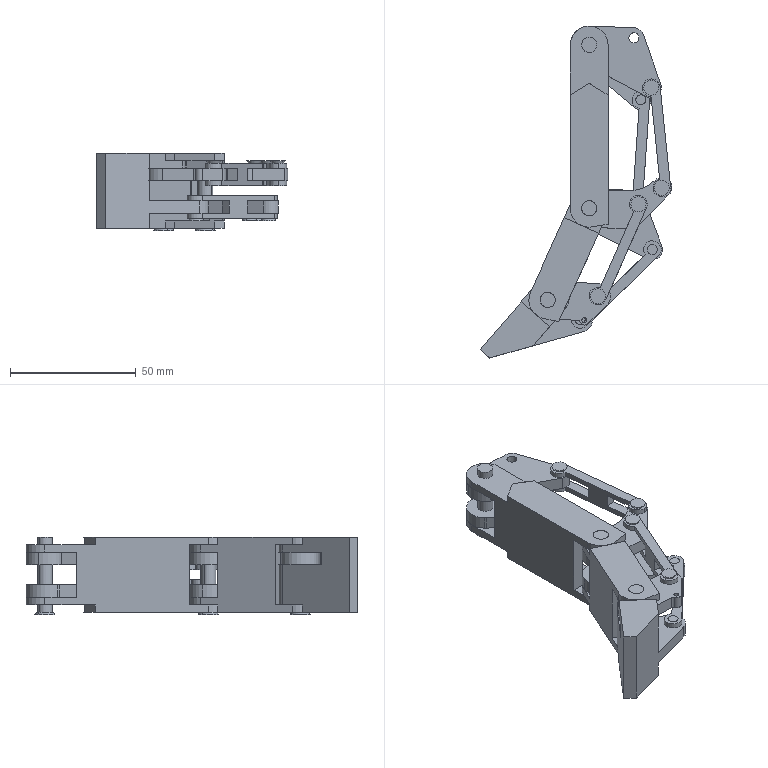Part | SolidWorks | features CompositeCurve 1 | 23 solids | 347 faces | box 76.237 x 131.963 x 31 mm | volume 53046 mm3 | cylinder 167 | plane 158 | cone 22 | commonest cylinder face diameters 4 x69 6 x37 7 x24 15 x19 8 x6 10 x6